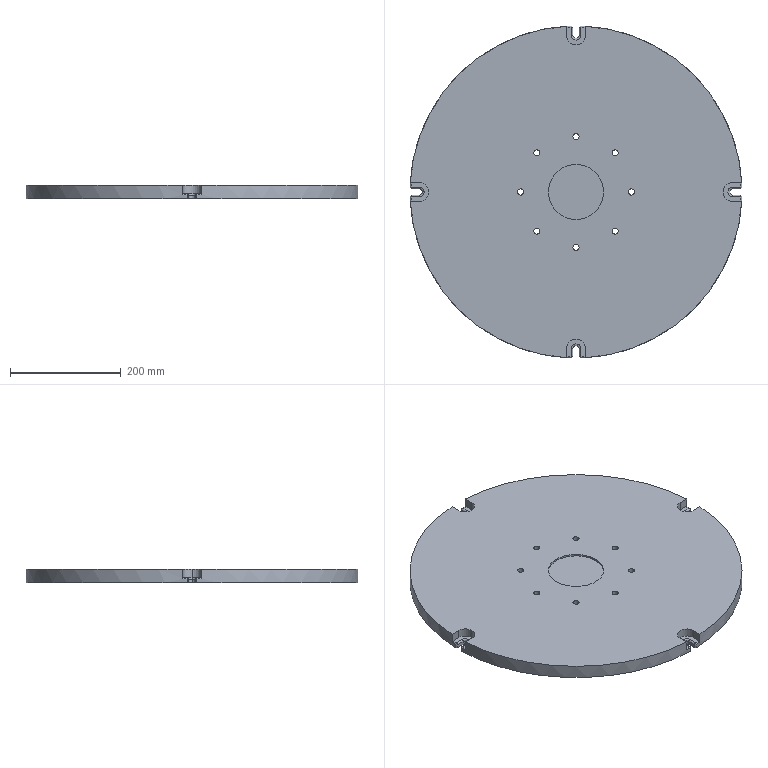Part | STEP file | Turntable | 1 solid | 92 faces | box 599.815 x 599.815 x 25 mm | volume 6952769 mm3 | cylinder 40 | plane 31 | spline 13 | cone 8 | commonest cylinder face diameters 11 x21 6 x8 34 x5 600 x4 100 x2